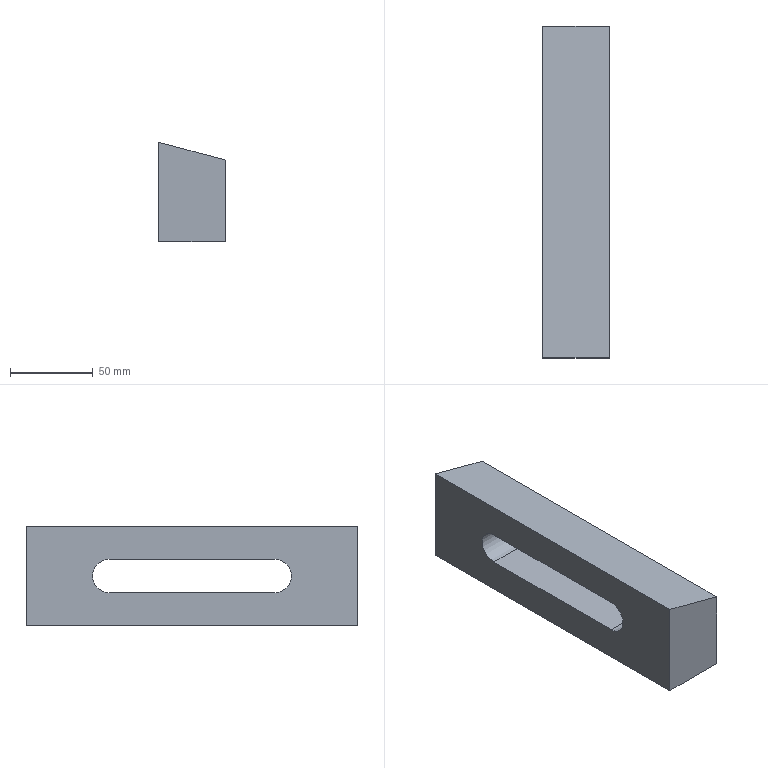Part | SolidWorks | features Extrusion 1, ICE 1 | 1 solid | 10 faces | box 40 x 200 x 60 mm | volume 344562 mm3 | plane 8 | cylinder 2 | commonest cylinder face diameters 20 x2
STEP:
#1=CARTESIAN_POINT('',(20.,200.,-10.718));
#2=VERTEX_POINT('',#1);
#3=CARTESIAN_POINT('',(20.,0.,-10.718));
#4=VERTEX_POINT('',#3);
#5=CARTESIAN_POINT('',(20.,200.,-10.718));
#6=DIRECTION('',(0.,-1.,0.));
#7=VECTOR('',#6,1000.);
#8=LINE('',#5,#7);
#9=EDGE_CURVE('',#2,#4,#8,.T.);
#10=ORIENTED_EDGE('',*,*,#9,.T.);
#11=CARTESIAN_POINT('',(20.,0.,-60.));
#12=VERTEX_POINT('',#11);
#13=CARTESIAN_POINT('',(20.,0.,0.));
#14=DIRECTION('',(0.,0.,-1.));
#15=VECTOR('',#14,1000.);
#16=LINE('',#13,#15);
#17=EDGE_CURVE('',#4,#12,#16,.T.);
#18=ORIENTED_EDGE('',*,*,#17,.T.);
#19=CARTESIAN_POINT('',(20.,200.,-60.));
#20=VERTEX_POINT('',#19);
#21=CARTESIAN_POINT('',(20.,0.,-60.));
#22=DIRECTION('',(0.,1.,0.));
#23=VECTOR('',#22,1000.);
#24=LINE('',#21,#23);
#25=EDGE_CURVE('',#12,#20,#24,.T.);
#26=ORIENTED_EDGE('',*,*,#25,.T.);
#27=CARTESIAN_POINT('',(20.,200.,-60.));
#28=DIRECTION('',(0.,0.,1.));
#29=VECTOR('',#28,1000.);
#30=LINE('',#27,#29);
#31=EDGE_CURVE('',#20,#2,#30,.T.);
#32=ORIENTED_EDGE('',*,*,#31,.T.);
#33=EDGE_LOOP('',(#10,#18,#26,#32));
#34=FACE_OUTER_BOUND('',#33,.T.);
#35=CARTESIAN_POINT('',(20.,50.,-40.));
#36=VERTEX_POINT('',#35);
#37=CARTESIAN_POINT('',(20.,150.,-40.));
#38=VERTEX_POINT('',#37);
#39=CARTESIAN_POINT('',(20.,50.,-40.));
#40=DIRECTION('',(0.,1.,0.));
#41=VECTOR('',#40,1000.);
#42=LINE('',#39,#41);
#43=EDGE_CURVE('',#36,#38,#42,.T.);
#44=ORIENTED_EDGE('',*,*,#43,.F.);
#45=CARTESIAN_POINT('',(20.,50.,-20.));
#46=VERTEX_POINT('',#45);
#47=CARTESIAN_POINT('',(20.,50.,-30.));
#48=DIRECTION('',(1.,0.,0.));
#49=DIRECTION('',(0.,0.,-1.));
#50=AXIS2_PLACEMENT_3D('',#47,#48,#49);
#51=CIRCLE('',#50,10.);
#52=EDGE_CURVE('',#46,#36,#51,.T.);
#53=ORIENTED_EDGE('',*,*,#52,.F.);
#54=CARTESIAN_POINT('',(20.,150.,-20.));
#55=VERTEX_POINT('',#54);
#56=CARTESIAN_POINT('',(20.,50.,-20.));
#57=DIRECTION('',(0.,-1.,0.));
#58=VECTOR('',#57,1000.);
#59=LINE('',#56,#58);
#60=EDGE_CURVE('',#55,#46,#59,.T.);
#61=ORIENTED_EDGE('',*,*,#60,.F.);
#62=CARTESIAN_POINT('',(20.,150.,-30.));
#63=DIRECTION('',(1.,0.,0.));
#64=DIRECTION('',(0.,0.,-1.));
#65=AXIS2_PLACEMENT_3D('',#62,#63,#64);
#66=CIRCLE('',#65,10.);
#67=EDGE_CURVE('',#38,#55,#66,.T.);
#68=ORIENTED_EDGE('',*,*,#67,.F.);
#69=EDGE_LOOP('',(#44,#53,#61,#68));
#70=FACE_BOUND('',#69,.T.);
#71=CARTESIAN_POINT('',(20.,0.,0.));
#72=DIRECTION('',(1.,0.,0.));
#73=DIRECTION('',(0.,0.,-1.));
#74=AXIS2_PLACEMENT_3D('',#71,#72,#73);
#75=PLANE('',#74);
#76=ADVANCED_FACE('',(#34,#70),#75,.T.);
#77=CARTESIAN_POINT('',(-20.,200.,0.));
#78=VERTEX_POINT('',#77);
#79=CARTESIAN_POINT('',(-20.,0.,0.));
#80=VERTEX_POINT('',#79);
#81=CARTESIAN_POINT('',(-20.,200.,0.));
#82=DIRECTION('',(0.,-1.,0.));
#83=VECTOR('',#82,1000.);
#84=LINE('',#81,#83);
#85=EDGE_CURVE('',#78,#80,#84,.T.);
#86=ORIENTED_EDGE('',*,*,#85,.F.);
#87=CARTESIAN_POINT('',(-20.,200.,-60.));
#88=VERTEX_POINT('',#87);
#89=CARTESIAN_POINT('',(-20.,200.,-60.));
#90=DIRECTION('',(0.,0.,1.));
#91=VECTOR('',#90,1000.);
#92=LINE('',#89,#91);
#93=EDGE_CURVE('',#88,#78,#92,.T.);
#94=ORIENTED_EDGE('',*,*,#93,.F.);
#95=CARTESIAN_POINT('',(-20.,0.,-60.));
#96=VERTEX_POINT('',#95);
#97=CARTESIAN_POINT('',(-20.,0.,-60.));
#98=DIRECTION('',(0.,1.,0.));
#99=VECTOR('',#98,1000.);
#100=LINE('',#97,#99);
#101=EDGE_CURVE('',#96,#88,#100,.T.);
#102=ORIENTED_EDGE('',*,*,#101,.F.);
#103=CARTESIAN_POINT('',(-20.,0.,0.));
#104=DIRECTION('',(0.,0.,-1.));
#105=VECTOR('',#104,1000.);
#106=LINE('',#103,#105);
#107=EDGE_CURVE('',#80,#96,#106,.T.);
#108=ORIENTED_EDGE('',*,*,#107,.F.);
#109=EDGE_LOOP('',(#86,#94,#102,#108));
#110=FACE_OUTER_BOUND('',#109,.T.);
#111=CARTESIAN_POINT('',(-20.,50.,-20.));
#112=VERTEX_POINT('',#111);
#113=CARTESIAN_POINT('',(-20.,50.,-40.));
#114=VERTEX_POINT('',#113);
#115=CARTESIAN_POINT('',(-20.,50.,-30.));
#116=DIRECTION('',(1.,0.,0.));
#117=DIRECTION('',(0.,0.,-1.));
#118=AXIS2_PLACEMENT_3D('',#115,#116,#117);
#119=CIRCLE('',#118,10.);
#120=EDGE_CURVE('',#112,#114,#119,.T.);
#121=ORIENTED_EDGE('',*,*,#120,.T.);
#122=CARTESIAN_POINT('',(-20.,150.,-40.));
#123=VERTEX_POINT('',#122);
#124=CARTESIAN_POINT('',(-20.,50.,-40.));
#125=DIRECTION('',(0.,1.,0.));
#126=VECTOR('',#125,1000.);
#127=LINE('',#124,#126);
#128=EDGE_CURVE('',#114,#123,#127,.T.);
#129=ORIENTED_EDGE('',*,*,#128,.T.);
#130=CARTESIAN_POINT('',(-20.,150.,-20.));
#131=VERTEX_POINT('',#130);
#132=CARTESIAN_POINT('',(-20.,150.,-30.));
#133=DIRECTION('',(1.,0.,0.));
#134=DIRECTION('',(0.,0.,-1.));
#135=AXIS2_PLACEMENT_3D('',#132,#133,#134);
#136=CIRCLE('',#135,10.);
#137=EDGE_CURVE('',#123,#131,#136,.T.);
#138=ORIENTED_EDGE('',*,*,#137,.T.);
#139=CARTESIAN_POINT('',(-20.,50.,-20.));
#140=DIRECTION('',(0.,-1.,0.));
#141=VECTOR('',#140,1000.);
#142=LINE('',#139,#141);
#143=EDGE_CURVE('',#131,#112,#142,.T.);
#144=ORIENTED_EDGE('',*,*,#143,.T.);
#145=EDGE_LOOP('',(#121,#129,#138,#144));
#146=FACE_BOUND('',#145,.T.);
#147=CARTESIAN_POINT('',(-20.,0.,0.));
#148=DIRECTION('',(1.,0.,0.));
#149=DIRECTION('',(0.,0.,-1.));
#150=AXIS2_PLACEMENT_3D('',#147,#148,#149);
#151=PLANE('',#150);
#152=ADVANCED_FACE('',(#110,#146),#151,.F.);
#153=ORIENTED_EDGE('',*,*,#17,.F.);
#154=CARTESIAN_POINT('',(-20.,0.,0.));
#155=DIRECTION('',(0.9659,0.,-0.2588));
#156=VECTOR('',#155,1000.);
#157=LINE('',#154,#156);
#158=EDGE_CURVE('',#80,#4,#157,.T.);
#159=ORIENTED_EDGE('',*,*,#158,.F.);
#160=ORIENTED_EDGE('',*,*,#107,.T.);
#161=CARTESIAN_POINT('',(20.,0.,-60.));
#162=DIRECTION('',(-1.,0.,0.));
#163=VECTOR('',#162,1000.);
#164=LINE('',#161,#163);
#165=EDGE_CURVE('',#12,#96,#164,.T.);
#166=ORIENTED_EDGE('',*,*,#165,.F.);
#167=EDGE_LOOP('',(#153,#159,#160,#166));
#168=FACE_OUTER_BOUND('',#167,.T.);
#169=CARTESIAN_POINT('',(20.,0.,0.));
#170=DIRECTION('',(0.,1.,0.));
#171=DIRECTION('',(0.,0.,1.));
#172=AXIS2_PLACEMENT_3D('',#169,#170,#171);
#173=PLANE('',#172);
#174=ADVANCED_FACE('',(#168),#173,.F.);
#175=ORIENTED_EDGE('',*,*,#101,.T.);
#176=CARTESIAN_POINT('',(20.,200.,-60.));
#177=DIRECTION('',(-1.,0.,0.));
#178=VECTOR('',#177,1000.);
#179=LINE('',#176,#178);
#180=EDGE_CURVE('',#20,#88,#179,.T.);
#181=ORIENTED_EDGE('',*,*,#180,.F.);
#182=ORIENTED_EDGE('',*,*,#25,.F.);
#183=ORIENTED_EDGE('',*,*,#165,.T.);
#184=EDGE_LOOP('',(#175,#181,#182,#183));
#185=FACE_OUTER_BOUND('',#184,.T.);
#186=CARTESIAN_POINT('',(20.,0.,-60.));
#187=DIRECTION('',(0.,0.,1.));
#188=DIRECTION('',(0.,-1.,0.));
#189=AXIS2_PLACEMENT_3D('',#186,#187,#188);
#190=PLANE('',#189);
#191=ADVANCED_FACE('',(#185),#190,.F.);
#192=ORIENTED_EDGE('',*,*,#93,.T.);
#193=CARTESIAN_POINT('',(-20.,200.,0.));
#194=DIRECTION('',(0.9659,0.,-0.2588));
#195=VECTOR('',#194,1000.);
#196=LINE('',#193,#195);
#197=EDGE_CURVE('',#78,#2,#196,.T.);
#198=ORIENTED_EDGE('',*,*,#197,.T.);
#199=ORIENTED_EDGE('',*,*,#31,.F.);
#200=ORIENTED_EDGE('',*,*,#180,.T.);
#201=EDGE_LOOP('',(#192,#198,#199,#200));
#202=FACE_OUTER_BOUND('',#201,.T.);
#203=CARTESIAN_POINT('',(20.,200.,-60.));
#204=DIRECTION('',(0.,-1.,0.));
#205=DIRECTION('',(0.,0.,-1.));
#206=AXIS2_PLACEMENT_3D('',#203,#204,#205);
#207=PLANE('',#206);
#208=ADVANCED_FACE('',(#202),#207,.F.);
#209=ORIENTED_EDGE('',*,*,#120,.F.);
#210=CARTESIAN_POINT('',(20.,50.,-20.));
#211=DIRECTION('',(-1.,0.,0.));
#212=VECTOR('',#211,1000.);
#213=LINE('',#210,#212);
#214=EDGE_CURVE('',#46,#112,#213,.T.);
#215=ORIENTED_EDGE('',*,*,#214,.F.);
#216=ORIENTED_EDGE('',*,*,#52,.T.);
#217=CARTESIAN_POINT('',(20.,50.,-40.));
#218=DIRECTION('',(-1.,0.,0.));
#219=VECTOR('',#218,1000.);
#220=LINE('',#217,#219);
#221=EDGE_CURVE('',#36,#114,#220,.T.);
#222=ORIENTED_EDGE('',*,*,#221,.T.);
#223=EDGE_LOOP('',(#209,#215,#216,#222));
#224=FACE_OUTER_BOUND('',#223,.T.);
#225=CARTESIAN_POINT('',(20.,50.,-30.));
#226=DIRECTION('',(-1.,0.,0.));
#227=DIRECTION('',(0.,0.,1.));
#228=AXIS2_PLACEMENT_3D('',#225,#226,#227);
#229=CYLINDRICAL_SURFACE('',#228,10.);
#230=ADVANCED_FACE('',(#224),#229,.F.);
#231=ORIENTED_EDGE('',*,*,#128,.F.);
#232=ORIENTED_EDGE('',*,*,#221,.F.);
#233=ORIENTED_EDGE('',*,*,#43,.T.);
#234=CARTESIAN_POINT('',(20.,150.,-40.));
#235=DIRECTION('',(-1.,0.,0.));
#236=VECTOR('',#235,1000.);
#237=LINE('',#234,#236);
#238=EDGE_CURVE('',#38,#123,#237,.T.);
#239=ORIENTED_EDGE('',*,*,#238,.T.);
#240=EDGE_LOOP('',(#231,#232,#233,#239));
#241=FACE_OUTER_BOUND('',#240,.T.);
#242=CARTESIAN_POINT('',(20.,50.,-40.));
#243=DIRECTION('',(0.,0.,1.));
#244=DIRECTION('',(1.,0.,0.));
#245=AXIS2_PLACEMENT_3D('',#242,#243,#244);
#246=PLANE('',#245);
#247=ADVANCED_FACE('',(#241),#246,.T.);
#248=ORIENTED_EDGE('',*,*,#137,.F.);
#249=ORIENTED_EDGE('',*,*,#238,.F.);
#250=ORIENTED_EDGE('',*,*,#67,.T.);
#251=CARTESIAN_POINT('',(20.,150.,-20.));
#252=DIRECTION('',(-1.,0.,0.));
#253=VECTOR('',#252,1000.);
#254=LINE('',#251,#253);
#255=EDGE_CURVE('',#55,#131,#254,.T.);
#256=ORIENTED_EDGE('',*,*,#255,.T.);
#257=EDGE_LOOP('',(#248,#249,#250,#256));
#258=FACE_OUTER_BOUND('',#257,.T.);
#259=CARTESIAN_POINT('',(20.,150.,-30.));
#260=DIRECTION('',(-1.,0.,0.));
#261=DIRECTION('',(0.,0.,1.));
#262=AXIS2_PLACEMENT_3D('',#259,#260,#261);
#263=CYLINDRICAL_SURFACE('',#262,10.);
#264=ADVANCED_FACE('',(#258),#263,.F.);
#265=ORIENTED_EDGE('',*,*,#143,.F.);
#266=ORIENTED_EDGE('',*,*,#255,.F.);
#267=ORIENTED_EDGE('',*,*,#60,.T.);
#268=ORIENTED_EDGE('',*,*,#214,.T.);
#269=EDGE_LOOP('',(#265,#266,#267,#268));
#270=FACE_OUTER_BOUND('',#269,.T.);
#271=CARTESIAN_POINT('',(20.,50.,-20.));
#272=DIRECTION('',(0.,0.,-1.));
#273=DIRECTION('',(-1.,0.,0.));
#274=AXIS2_PLACEMENT_3D('',#271,#272,#273);
#275=PLANE('',#274);
#276=ADVANCED_FACE('',(#270),#275,.T.);
#277=ORIENTED_EDGE('',*,*,#158,.T.);
#278=ORIENTED_EDGE('',*,*,#9,.F.);
#279=ORIENTED_EDGE('',*,*,#197,.F.);
#280=ORIENTED_EDGE('',*,*,#85,.T.);
#281=EDGE_LOOP('',(#277,#278,#279,#280));
#282=FACE_OUTER_BOUND('',#281,.T.);
#283=CARTESIAN_POINT('',(-20.,200.,0.));
#284=DIRECTION('',(-0.2588,0.,-0.9659));
#285=DIRECTION('',(-0.9659,0.,0.2588));
#286=AXIS2_PLACEMENT_3D('',#283,#284,#285);
#287=PLANE('',#286);
#288=ADVANCED_FACE('',(#282),#287,.F.);
#289=CLOSED_SHELL('',(#76,#152,#174,#191,#208,#230,#247,#264,#276,#288));
#290=MANIFOLD_SOLID_BREP('',#289);
#291=CARTESIAN_POINT('',(0.,0.,0.));
#292=DIRECTION('',(0.,0.,1.));
#293=DIRECTION('',(1.,0.,0.));
#294=AXIS2_PLACEMENT_3D('',#291,#292,#293);
#295=(LENGTH_UNIT()NAMED_UNIT(*)SI_UNIT(.MILLI.,.METRE.));
#296=UNCERTAINTY_MEASURE_WITH_UNIT(LENGTH_MEASURE(0.00001),#295,'','');
#297=(NAMED_UNIT(*)PLANE_ANGLE_UNIT()SI_UNIT($,.RADIAN.));
#298=(NAMED_UNIT(*)SI_UNIT($,.STERADIAN.)SOLID_ANGLE_UNIT());
#299=(GEOMETRIC_REPRESENTATION_CONTEXT(3)GLOBAL_UNCERTAINTY_ASSIGNED_CONTEXT((#296))GLOBAL_UNIT_ASSIGNED_CONTEXT((#295,#297,#298))REPRESENTATION_CONTEXT('',''));
#300=ADVANCED_BREP_SHAPE_REPRESENTATION('',(#290,#294),#299);